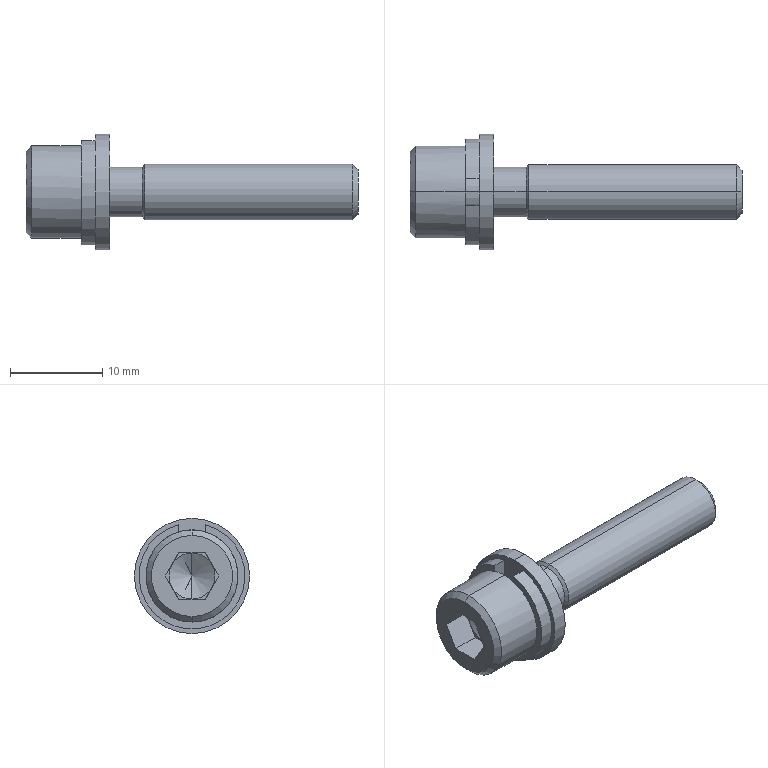Part | STEP file | 0244_016_SCBS6-30 | 1 solid | 39 faces | box 36 x 12.5 x 12.5 mm | volume 1452 mm3 | plane 20 | cylinder 11 | cone 8 | commonest cylinder face diameters 6 x4 5.386 x2 10 x2 12.5 x2 11.5 x1